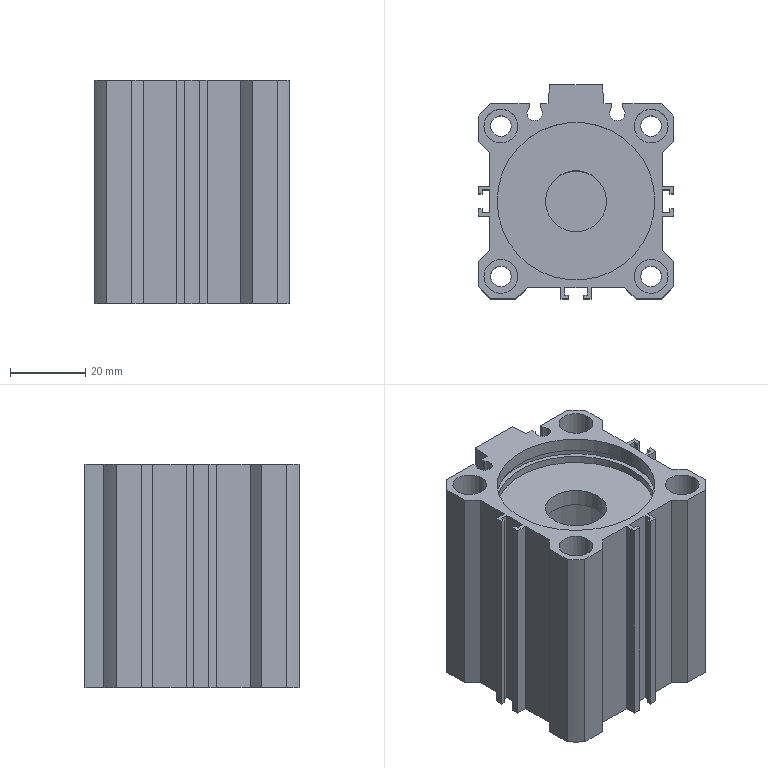Part | STEP file | CQ2B40-30D_CQ2Tube | 1 solid | 144 faces | box 52 x 57 x 59.5 mm | volume 79624 mm3 | plane 82 | cylinder 54 | cone 8 | commonest cylinder face diameters 9 x16 5.5 x8 4.15 x6 7.9 x4 16.25 x4 42 x4